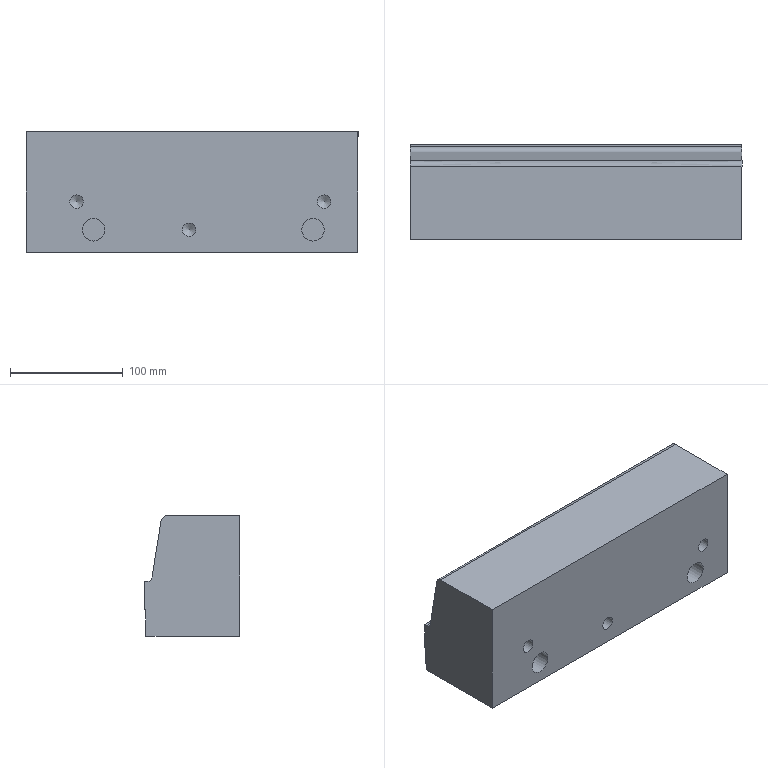Part | NX | features solid 2 | 1 solid | 22 faces | box 295 x 84.706 x 107.133 mm | volume 2449050 mm3 | plane 9 | cylinder 6 | spline 4 | cone 3 | commonest cylinder face diameters 12 x3 20 x2 10 x1
STEP:
#1=CARTESIAN_POINT('',(75.,-76.708,-50.));
#2=VERTEX_POINT('',#1);
#3=CARTESIAN_POINT('',(370.,-76.709,-50.));
#4=VERTEX_POINT('',#3);
#5=CARTESIAN_POINT('',(75.,-76.708,-50.));
#6=CARTESIAN_POINT('',(173.333,-76.71,-50.));
#7=CARTESIAN_POINT('',(271.667,-76.709,-50.));
#8=CARTESIAN_POINT('',(370.,-76.709,-50.));
#9=B_SPLINE_CURVE_WITH_KNOTS('',3,(#5,#6,#7,#8),.UNSPECIFIED.,.F.,.F.,(4,4),(0.1723,0.4673),.UNSPECIFIED.);
#10=EDGE_CURVE('',#2,#4,#9,.T.);
#11=ORIENTED_EDGE('',*,*,#10,.F.);
#12=CARTESIAN_POINT('',(75.,-76.507,-26.5));
#13=VERTEX_POINT('',#12);
#14=CARTESIAN_POINT('',(75.,-76.608,-38.267));
#15=DIRECTION('',(0.,-0.008536,-1.));
#16=VECTOR('',#15,1000.);
#17=LINE('',#14,#16);
#18=EDGE_CURVE('',#2,#13,#17,.F.);
#19=ORIENTED_EDGE('',*,*,#18,.T.);
#20=CARTESIAN_POINT('',(370.,-76.508,-26.5));
#21=VERTEX_POINT('',#20);
#22=CARTESIAN_POINT('',(75.,-76.507,-26.5));
#23=CARTESIAN_POINT('',(173.333,-76.509,-26.5));
#24=CARTESIAN_POINT('',(271.667,-76.508,-26.5));
#25=CARTESIAN_POINT('',(370.,-76.508,-26.5));
#26=B_SPLINE_CURVE_WITH_KNOTS('',3,(#22,#23,#24,#25),.UNSPECIFIED.,.F.,.F.,(4,4),(0.1378,0.4328),.UNSPECIFIED.);
#27=EDGE_CURVE('',#13,#21,#26,.T.);
#28=ORIENTED_EDGE('',*,*,#27,.T.);
#29=CARTESIAN_POINT('',(370.,-76.608,-38.267));
#30=DIRECTION('',(0.,-0.008536,-1.));
#31=VECTOR('',#30,1000.);
#32=LINE('',#29,#31);
#33=EDGE_CURVE('',#4,#21,#32,.F.);
#34=ORIENTED_EDGE('',*,*,#33,.F.);
#35=EDGE_LOOP('',(#11,#19,#28,#34));
#36=FACE_BOUND('',#35,.T.);
#37=CARTESIAN_POINT('',(75.,-76.507,-26.5));
#38=CARTESIAN_POINT('',(75.,-76.708,-50.));
#39=CARTESIAN_POINT('',(173.333,-76.509,-26.5));
#40=CARTESIAN_POINT('',(173.333,-76.71,-50.));
#41=CARTESIAN_POINT('',(271.667,-76.508,-26.5));
#42=CARTESIAN_POINT('',(271.667,-76.709,-50.));
#43=CARTESIAN_POINT('',(370.,-76.508,-26.5));
#44=CARTESIAN_POINT('',(370.,-76.709,-50.));
#45=B_SPLINE_SURFACE_WITH_KNOTS('',3,1,((#37,#38),(#39,#40),(#41,#42),(#43,#44)),.SURF_OF_LINEAR_EXTRUSION.,.F.,.F.,.F.,(4,4),(2,2),(0.5716,0.7876),(0.,1.),.PIECEWISE_BEZIER_KNOTS.);
#46=ADVANCED_FACE('',(#36),#45,.T.);
#47=ORIENTED_EDGE('',*,*,#33,.T.);
#48=CARTESIAN_POINT('',(370.,-75.295,-26.51));
#49=VERTEX_POINT('',#48);
#50=CARTESIAN_POINT('',(370.,-75.914,-26.505));
#51=DIRECTION('',(0.,-1.,0.008536));
#52=VECTOR('',#51,1000.);
#53=LINE('',#50,#52);
#54=EDGE_CURVE('',#49,#21,#53,.T.);
#55=ORIENTED_EDGE('',*,*,#54,.F.);
#56=CARTESIAN_POINT('',(370.,-75.295,-1.509));
#57=VERTEX_POINT('',#56);
#58=CARTESIAN_POINT('',(370.,-75.295,-14.009));
#59=DIRECTION('',(0.,0.,-1.));
#60=VECTOR('',#59,1000.);
#61=LINE('',#58,#60);
#62=EDGE_CURVE('',#57,#49,#61,.T.);
#63=ORIENTED_EDGE('',*,*,#62,.F.);
#64=CARTESIAN_POINT('',(370.,-77.294,-1.492));
#65=VERTEX_POINT('',#64);
#66=CARTESIAN_POINT('',(370.,47.797,-2.56));
#67=DIRECTION('',(0.,1.,-0.008536));
#68=VECTOR('',#67,1000.);
#69=LINE('',#66,#68);
#70=EDGE_CURVE('',#65,#57,#69,.T.);
#71=ORIENTED_EDGE('',*,*,#70,.F.);
#72=CARTESIAN_POINT('',(370.,-82.189,2.72));
#73=VERTEX_POINT('',#72);
#74=CARTESIAN_POINT('',(370.,-77.252,3.508));
#75=DIRECTION('',(-1.,0.,0.));
#76=DIRECTION('',(0.,0.,1.));
#77=AXIS2_PLACEMENT_3D('',#74,#75,#76);
#78=CIRCLE('',#77,5.);
#79=EDGE_CURVE('',#73,#65,#78,.F.);
#80=ORIENTED_EDGE('',*,*,#79,.F.);
#81=CARTESIAN_POINT('',(370.,-90.197,52.92));
#82=VERTEX_POINT('',#81);
#83=CARTESIAN_POINT('',(370.,-86.499,29.736));
#84=DIRECTION('',(0.,0.1575,-0.9875));
#85=VECTOR('',#84,1000.);
#86=LINE('',#83,#85);
#87=EDGE_CURVE('',#82,#73,#86,.T.);
#88=ORIENTED_EDGE('',*,*,#87,.F.);
#89=CARTESIAN_POINT('',(370.,-95.134,57.133));
#90=VERTEX_POINT('',#89);
#91=CARTESIAN_POINT('',(370.,-95.134,52.133));
#92=DIRECTION('',(-1.,0.,0.));
#93=DIRECTION('',(0.,0.,1.));
#94=AXIS2_PLACEMENT_3D('',#91,#92,#93);
#95=CIRCLE('',#94,5.);
#96=EDGE_CURVE('',#82,#90,#95,.F.);
#97=ORIENTED_EDGE('',*,*,#96,.T.);
#98=CARTESIAN_POINT('',(370.,-160.,57.133));
#99=VERTEX_POINT('',#98);
#100=CARTESIAN_POINT('',(370.,-90.869,57.133));
#101=DIRECTION('',(0.,-1.,0.));
#102=VECTOR('',#101,1000.);
#103=LINE('',#100,#102);
#104=EDGE_CURVE('',#90,#99,#103,.T.);
#105=ORIENTED_EDGE('',*,*,#104,.T.);
#106=CARTESIAN_POINT('',(370.,-160.,-50.));
#107=VERTEX_POINT('',#106);
#108=CARTESIAN_POINT('',(370.,-160.,200.));
#109=DIRECTION('',(0.,0.,1.));
#110=VECTOR('',#109,1000.);
#111=LINE('',#108,#110);
#112=EDGE_CURVE('',#107,#99,#111,.T.);
#113=ORIENTED_EDGE('',*,*,#112,.F.);
#114=CARTESIAN_POINT('',(370.,361.,-50.));
#115=DIRECTION('',(0.,-1.,0.));
#116=VECTOR('',#115,1000.);
#117=LINE('',#114,#116);
#118=EDGE_CURVE('',#107,#4,#117,.F.);
#119=ORIENTED_EDGE('',*,*,#118,.T.);
#120=EDGE_LOOP('',(#47,#55,#63,#71,#80,#88,#97,#105,#113,#119));
#121=FACE_BOUND('',#120,.T.);
#122=CARTESIAN_POINT('',(370.,361.,0.));
#123=DIRECTION('',(-1.,0.,0.));
#124=DIRECTION('',(0.,0.,1.));
#125=AXIS2_PLACEMENT_3D('',#122,#123,#124);
#126=PLANE('',#125);
#127=ADVANCED_FACE('',(#121),#126,.F.);
#128=CARTESIAN_POINT('',(75.,-160.,-50.));
#129=VERTEX_POINT('',#128);
#130=CARTESIAN_POINT('',(75.,-159.,-50.));
#131=DIRECTION('',(0.,1.,0.));
#132=VECTOR('',#131,1000.);
#133=LINE('',#130,#132);
#134=EDGE_CURVE('',#129,#2,#133,.T.);
#135=ORIENTED_EDGE('',*,*,#134,.T.);
#136=ORIENTED_EDGE('',*,*,#10,.T.);
#137=ORIENTED_EDGE('',*,*,#118,.F.);
#138=CARTESIAN_POINT('',(-571.479,-160.,-50.));
#139=DIRECTION('',(1.,0.,0.));
#140=VECTOR('',#139,1000.);
#141=LINE('',#138,#140);
#142=EDGE_CURVE('',#129,#107,#141,.T.);
#143=ORIENTED_EDGE('',*,*,#142,.F.);
#144=EDGE_LOOP('',(#135,#136,#137,#143));
#145=FACE_BOUND('',#144,.T.);
#146=CARTESIAN_POINT('',(-571.479,-74.471,-50.));
#147=DIRECTION('',(0.,0.,-1.));
#148=DIRECTION('',(-1.,0.,0.));
#149=AXIS2_PLACEMENT_3D('',#146,#147,#148);
#150=PLANE('',#149);
#151=ADVANCED_FACE('',(#145),#150,.T.);
#152=ORIENTED_EDGE('',*,*,#142,.T.);
#153=ORIENTED_EDGE('',*,*,#112,.T.);
#154=CARTESIAN_POINT('',(75.,-160.,57.133));
#155=VERTEX_POINT('',#154);
#156=CARTESIAN_POINT('',(-705.,-160.,57.133));
#157=DIRECTION('',(1.,0.,0.));
#158=VECTOR('',#157,1000.);
#159=LINE('',#156,#158);
#160=EDGE_CURVE('',#155,#99,#159,.T.);
#161=ORIENTED_EDGE('',*,*,#160,.F.);
#162=CARTESIAN_POINT('',(75.,-160.,200.));
#163=DIRECTION('',(0.,0.,1.));
#164=VECTOR('',#163,1000.);
#165=LINE('',#162,#164);
#166=EDGE_CURVE('',#129,#155,#165,.T.);
#167=ORIENTED_EDGE('',*,*,#166,.F.);
#168=EDGE_LOOP('',(#152,#153,#161,#167));
#169=FACE_BOUND('',#168,.T.);
#170=CARTESIAN_POINT('',(340.,-160.,1.));
#171=VERTEX_POINT('',#170);
#172=CARTESIAN_POINT('',(340.,-160.,-5.));
#173=DIRECTION('',(0.,1.,0.));
#174=DIRECTION('',(0.,0.,1.));
#175=AXIS2_PLACEMENT_3D('',#172,#173,#174);
#176=CIRCLE('',#175,6.);
#177=EDGE_CURVE('',#171,#171,#176,.T.);
#178=ORIENTED_EDGE('',*,*,#177,.T.);
#179=EDGE_LOOP('',(#178));
#180=FACE_BOUND('',#179,.T.);
#181=CARTESIAN_POINT('',(220.,-160.,-24.));
#182=VERTEX_POINT('',#181);
#183=CARTESIAN_POINT('',(220.,-160.,-30.));
#184=DIRECTION('',(0.,1.,0.));
#185=DIRECTION('',(0.,0.,1.));
#186=AXIS2_PLACEMENT_3D('',#183,#184,#185);
#187=CIRCLE('',#186,6.);
#188=EDGE_CURVE('',#182,#182,#187,.T.);
#189=ORIENTED_EDGE('',*,*,#188,.T.);
#190=EDGE_LOOP('',(#189));
#191=FACE_BOUND('',#190,.T.);
#192=CARTESIAN_POINT('',(120.,-160.,1.));
#193=VERTEX_POINT('',#192);
#194=CARTESIAN_POINT('',(120.,-160.,-5.));
#195=DIRECTION('',(0.,1.,0.));
#196=DIRECTION('',(0.,0.,1.));
#197=AXIS2_PLACEMENT_3D('',#194,#195,#196);
#198=CIRCLE('',#197,6.);
#199=EDGE_CURVE('',#193,#193,#198,.T.);
#200=ORIENTED_EDGE('',*,*,#199,.T.);
#201=EDGE_LOOP('',(#200));
#202=FACE_BOUND('',#201,.T.);
#203=CARTESIAN_POINT('',(330.,-160.,-20.));
#204=VERTEX_POINT('',#203);
#205=CARTESIAN_POINT('',(330.,-160.,-30.));
#206=DIRECTION('',(0.,1.,0.));
#207=DIRECTION('',(0.,0.,1.));
#208=AXIS2_PLACEMENT_3D('',#205,#206,#207);
#209=CIRCLE('',#208,10.);
#210=EDGE_CURVE('',#204,#204,#209,.T.);
#211=ORIENTED_EDGE('',*,*,#210,.T.);
#212=EDGE_LOOP('',(#211));
#213=FACE_BOUND('',#212,.T.);
#214=CARTESIAN_POINT('',(135.,-160.,-20.));
#215=VERTEX_POINT('',#214);
#216=CARTESIAN_POINT('',(135.,-160.,-30.));
#217=DIRECTION('',(0.,1.,0.));
#218=DIRECTION('',(0.,0.,1.));
#219=AXIS2_PLACEMENT_3D('',#216,#217,#218);
#220=CIRCLE('',#219,10.);
#221=EDGE_CURVE('',#215,#215,#220,.T.);
#222=ORIENTED_EDGE('',*,*,#221,.T.);
#223=EDGE_LOOP('',(#222));
#224=FACE_BOUND('',#223,.T.);
#225=CARTESIAN_POINT('',(-705.,-160.,200.));
#226=DIRECTION('',(0.,1.,0.));
#227=DIRECTION('',(0.,0.,1.));
#228=AXIS2_PLACEMENT_3D('',#225,#226,#227);
#229=PLANE('',#228);
#230=ADVANCED_FACE('',(#169,#180,#191,#202,#213,#224),#229,.F.);
#231=ORIENTED_EDGE('',*,*,#96,.F.);
#232=CARTESIAN_POINT('',(75.,-90.197,52.92));
#233=VERTEX_POINT('',#232);
#234=CARTESIAN_POINT('',(75.,-90.197,52.92));
#235=CARTESIAN_POINT('',(173.333,-90.197,52.92));
#236=CARTESIAN_POINT('',(271.667,-90.197,52.92));
#237=CARTESIAN_POINT('',(370.,-90.197,52.92));
#238=B_SPLINE_CURVE_WITH_KNOTS('',3,(#234,#235,#236,#237),.UNSPECIFIED.,.F.,.F.,(4,4),(0.2731,0.5681),.UNSPECIFIED.);
#239=EDGE_CURVE('',#233,#82,#238,.T.);
#240=ORIENTED_EDGE('',*,*,#239,.F.);
#241=CARTESIAN_POINT('',(75.,-95.134,57.133));
#242=VERTEX_POINT('',#241);
#243=CARTESIAN_POINT('',(75.,-95.134,52.133));
#244=DIRECTION('',(-1.,0.,0.));
#245=DIRECTION('',(0.,0.,1.));
#246=AXIS2_PLACEMENT_3D('',#243,#244,#245);
#247=CIRCLE('',#246,5.);
#248=EDGE_CURVE('',#233,#242,#247,.F.);
#249=ORIENTED_EDGE('',*,*,#248,.T.);
#250=CARTESIAN_POINT('',(370.,-95.134,57.133));
#251=CARTESIAN_POINT('',(271.667,-95.134,57.133));
#252=CARTESIAN_POINT('',(173.333,-95.134,57.133));
#253=CARTESIAN_POINT('',(75.,-95.134,57.133));
#254=B_SPLINE_CURVE_WITH_KNOTS('',3,(#250,#251,#252,#253),.UNSPECIFIED.,.F.,.F.,(4,4),(0.3736,0.6686),.UNSPECIFIED.);
#255=EDGE_CURVE('',#90,#242,#254,.T.);
#256=ORIENTED_EDGE('',*,*,#255,.F.);
#257=EDGE_LOOP('',(#231,#240,#249,#256));
#258=FACE_BOUND('',#257,.T.);
#259=CARTESIAN_POINT('',(370.,-90.197,52.92));
#260=CARTESIAN_POINT('',(370.,-90.869,57.133));
#261=CARTESIAN_POINT('',(370.,-95.134,57.133));
#262=CARTESIAN_POINT('',(271.667,-90.197,52.92));
#263=CARTESIAN_POINT('',(271.667,-90.869,57.133));
#264=CARTESIAN_POINT('',(271.667,-95.134,57.133));
#265=CARTESIAN_POINT('',(173.333,-90.197,52.92));
#266=CARTESIAN_POINT('',(173.333,-90.869,57.133));
#267=CARTESIAN_POINT('',(173.333,-95.134,57.133));
#268=CARTESIAN_POINT('',(75.,-90.197,52.92));
#269=CARTESIAN_POINT('',(75.,-90.869,57.133));
#270=CARTESIAN_POINT('',(75.,-95.134,57.133));
#271=(BOUNDED_SURFACE()B_SPLINE_SURFACE(3,2,((#259,#260,#261),(#262,#263,#264),(#265,#266,#267),(#268,#269,#270)),.UNSPECIFIED.,.F.,.F.,.F.)B_SPLINE_SURFACE_WITH_KNOTS((4,4),(3,3),(0.4893,0.7843),(0.,1.),.PIECEWISE_BEZIER_KNOTS.)GEOMETRIC_REPRESENTATION_ITEM()RATIONAL_B_SPLINE_SURFACE(((1.,0.7608,1.),(1.,0.7608,1.),(1.,0.7608,1.),(1.,0.7608,1.)))REPRESENTATION_ITEM('')SURFACE());
#272=ADVANCED_FACE('',(#258),#271,.T.);
#273=ORIENTED_EDGE('',*,*,#239,.T.);
#274=ORIENTED_EDGE('',*,*,#87,.T.);
#275=CARTESIAN_POINT('',(75.,-82.189,2.72));
#276=VERTEX_POINT('',#275);
#277=CARTESIAN_POINT('',(75.,-82.189,2.72));
#278=CARTESIAN_POINT('',(173.333,-82.189,2.72));
#279=CARTESIAN_POINT('',(271.667,-82.189,2.72));
#280=CARTESIAN_POINT('',(370.,-82.189,2.72));
#281=B_SPLINE_CURVE_WITH_KNOTS('',3,(#277,#278,#279,#280),.UNSPECIFIED.,.F.,.F.,(4,4),(0.3113,0.6615),.UNSPECIFIED.);
#282=EDGE_CURVE('',#276,#73,#281,.T.);
#283=ORIENTED_EDGE('',*,*,#282,.F.);
#284=CARTESIAN_POINT('',(75.,-86.499,29.736));
#285=DIRECTION('',(0.,0.1575,-0.9875));
#286=VECTOR('',#285,1000.);
#287=LINE('',#284,#286);
#288=EDGE_CURVE('',#233,#276,#287,.T.);
#289=ORIENTED_EDGE('',*,*,#288,.F.);
#290=EDGE_LOOP('',(#273,#274,#283,#289));
#291=FACE_BOUND('',#290,.T.);
#292=CARTESIAN_POINT('',(808.196,-81.695,-0.3814));
#293=CARTESIAN_POINT('',(-199.284,-81.695,-0.3814));
#294=CARTESIAN_POINT('',(808.196,-91.303,59.853));
#295=CARTESIAN_POINT('',(-199.284,-91.303,59.853));
#296=B_SPLINE_SURFACE_WITH_KNOTS('',1,1,((#292,#293),(#294,#295)),.PLANE_SURF.,.F.,.F.,.F.,(2,2),(2,2),(-0.06964,1.283),(-0.1722,1.),.UNSPECIFIED.);
#297=ADVANCED_FACE('',(#291),#296,.F.);
#298=ORIENTED_EDGE('',*,*,#282,.T.);
#299=ORIENTED_EDGE('',*,*,#79,.T.);
#300=CARTESIAN_POINT('',(75.,-77.294,-1.492));
#301=VERTEX_POINT('',#300);
#302=CARTESIAN_POINT('',(370.,-77.294,-1.492));
#303=CARTESIAN_POINT('',(271.667,-77.294,-1.492));
#304=CARTESIAN_POINT('',(173.333,-77.294,-1.492));
#305=CARTESIAN_POINT('',(75.,-77.294,-1.492));
#306=B_SPLINE_CURVE_WITH_KNOTS('',3,(#302,#303,#304,#305),.UNSPECIFIED.,.F.,.F.,(4,4),(0.3388,0.6888),.UNSPECIFIED.);
#307=EDGE_CURVE('',#65,#301,#306,.T.);
#308=ORIENTED_EDGE('',*,*,#307,.T.);
#309=CARTESIAN_POINT('',(75.,-77.252,3.508));
#310=DIRECTION('',(-1.,0.,0.));
#311=DIRECTION('',(0.,0.,1.));
#312=AXIS2_PLACEMENT_3D('',#309,#310,#311);
#313=CIRCLE('',#312,5.);
#314=EDGE_CURVE('',#276,#301,#313,.F.);
#315=ORIENTED_EDGE('',*,*,#314,.F.);
#316=EDGE_LOOP('',(#298,#299,#308,#315));
#317=FACE_BOUND('',#316,.T.);
#318=CARTESIAN_POINT('',(6000655.556,-77.252,3.508));
#319=DIRECTION('',(-1.,0.,0.));
#320=DIRECTION('',(0.,-0.1575,0.9875));
#321=AXIS2_PLACEMENT_3D('',#318,#319,#320);
#322=CYLINDRICAL_SURFACE('',#321,5.);
#323=ADVANCED_FACE('',(#317),#322,.F.);
#324=ORIENTED_EDGE('',*,*,#307,.F.);
#325=ORIENTED_EDGE('',*,*,#70,.T.);
#326=CARTESIAN_POINT('',(75.,-75.294,-1.509));
#327=VERTEX_POINT('',#326);
#328=CARTESIAN_POINT('',(75.,-75.294,-1.509));
#329=CARTESIAN_POINT('',(173.333,-75.295,-1.509));
#330=CARTESIAN_POINT('',(271.667,-75.295,-1.509));
#331=CARTESIAN_POINT('',(370.,-75.295,-1.509));
#332=B_SPLINE_CURVE_WITH_KNOTS('',3,(#328,#329,#330,#331),.UNSPECIFIED.,.F.,.F.,(4,4),(0.4725,0.7675),.UNSPECIFIED.);
#333=EDGE_CURVE('',#327,#57,#332,.T.);
#334=ORIENTED_EDGE('',*,*,#333,.F.);
#335=CARTESIAN_POINT('',(75.,47.797,-2.56));
#336=DIRECTION('',(0.,1.,-0.008536));
#337=VECTOR('',#336,1000.);
#338=LINE('',#335,#337);
#339=EDGE_CURVE('',#301,#327,#338,.T.);
#340=ORIENTED_EDGE('',*,*,#339,.F.);
#341=EDGE_LOOP('',(#324,#325,#334,#340));
#342=FACE_BOUND('',#341,.T.);
#343=CARTESIAN_POINT('',(35.495,47.797,-2.56));
#344=DIRECTION('',(0.,-0.008536,-1.));
#345=DIRECTION('',(0.,-1.,0.008536));
#346=AXIS2_PLACEMENT_3D('',#343,#344,#345);
#347=PLANE('',#346);
#348=ADVANCED_FACE('',(#342),#347,.F.);
#349=ORIENTED_EDGE('',*,*,#333,.T.);
#350=ORIENTED_EDGE('',*,*,#62,.T.);
#351=CARTESIAN_POINT('',(75.,-75.294,-26.51));
#352=VERTEX_POINT('',#351);
#353=CARTESIAN_POINT('',(370.,-75.295,-26.51));
#354=CARTESIAN_POINT('',(271.667,-75.295,-26.51));
#355=CARTESIAN_POINT('',(173.333,-75.295,-26.51));
#356=CARTESIAN_POINT('',(75.,-75.294,-26.51));
#357=B_SPLINE_CURVE_WITH_KNOTS('',3,(#353,#354,#355,#356),.UNSPECIFIED.,.F.,.F.,(4,4),(0.29,0.585),.UNSPECIFIED.);
#358=EDGE_CURVE('',#49,#352,#357,.T.);
#359=ORIENTED_EDGE('',*,*,#358,.T.);
#360=CARTESIAN_POINT('',(75.,-75.294,-14.008));
#361=DIRECTION('',(0.,0.,-1.));
#362=VECTOR('',#361,1000.);
#363=LINE('',#360,#362);
#364=EDGE_CURVE('',#327,#352,#363,.T.);
#365=ORIENTED_EDGE('',*,*,#364,.F.);
#366=EDGE_LOOP('',(#349,#350,#359,#365));
#367=FACE_BOUND('',#366,.T.);
#368=CARTESIAN_POINT('',(370.,-75.295,-1.509));
#369=CARTESIAN_POINT('',(370.,-75.295,-26.51));
#370=CARTESIAN_POINT('',(271.667,-75.295,-1.509));
#371=CARTESIAN_POINT('',(271.667,-75.295,-26.51));
#372=CARTESIAN_POINT('',(173.333,-75.295,-1.509));
#373=CARTESIAN_POINT('',(173.333,-75.295,-26.51));
#374=CARTESIAN_POINT('',(75.,-75.294,-1.509));
#375=CARTESIAN_POINT('',(75.,-75.294,-26.51));
#376=B_SPLINE_SURFACE_WITH_KNOTS('',3,1,((#368,#369),(#370,#371),(#372,#373),(#374,#375)),.SURF_OF_LINEAR_EXTRUSION.,.F.,.F.,.F.,(4,4),(2,2),(0.2124,0.4284),(0.,1.),.PIECEWISE_BEZIER_KNOTS.);
#377=ADVANCED_FACE('',(#367),#376,.F.);
#378=ORIENTED_EDGE('',*,*,#27,.F.);
#379=CARTESIAN_POINT('',(75.,-75.914,-26.505));
#380=DIRECTION('',(0.,-1.,0.008536));
#381=VECTOR('',#380,1000.);
#382=LINE('',#379,#381);
#383=EDGE_CURVE('',#352,#13,#382,.T.);
#384=ORIENTED_EDGE('',*,*,#383,.F.);
#385=ORIENTED_EDGE('',*,*,#358,.F.);
#386=ORIENTED_EDGE('',*,*,#54,.T.);
#387=EDGE_LOOP('',(#378,#384,#385,#386));
#388=FACE_BOUND('',#387,.T.);
#389=CARTESIAN_POINT('',(-437.652,-75.914,-26.505));
#390=DIRECTION('',(0.,0.008536,1.));
#391=DIRECTION('',(0.,-1.,0.008536));
#392=AXIS2_PLACEMENT_3D('',#389,#390,#391);
#393=PLANE('',#392);
#394=ADVANCED_FACE('',(#388),#393,.F.);
#395=ORIENTED_EDGE('',*,*,#383,.T.);
#396=ORIENTED_EDGE('',*,*,#18,.F.);
#397=ORIENTED_EDGE('',*,*,#134,.F.);
#398=ORIENTED_EDGE('',*,*,#166,.T.);
#399=CARTESIAN_POINT('',(75.,-90.869,57.133));
#400=DIRECTION('',(0.,-1.,0.));
#401=VECTOR('',#400,1000.);
#402=LINE('',#399,#401);
#403=EDGE_CURVE('',#242,#155,#402,.T.);
#404=ORIENTED_EDGE('',*,*,#403,.F.);
#405=ORIENTED_EDGE('',*,*,#248,.F.);
#406=ORIENTED_EDGE('',*,*,#288,.T.);
#407=ORIENTED_EDGE('',*,*,#314,.T.);
#408=ORIENTED_EDGE('',*,*,#339,.T.);
#409=ORIENTED_EDGE('',*,*,#364,.T.);
#410=EDGE_LOOP('',(#395,#396,#397,#398,#404,#405,#406,#407,#408,#409));
#411=FACE_BOUND('',#410,.T.);
#412=CARTESIAN_POINT('',(75.,361.,0.));
#413=DIRECTION('',(-1.,0.,0.));
#414=DIRECTION('',(0.,0.,1.));
#415=AXIS2_PLACEMENT_3D('',#412,#413,#414);
#416=PLANE('',#415);
#417=ADVANCED_FACE('',(#411),#416,.T.);
#418=ORIENTED_EDGE('',*,*,#104,.F.);
#419=ORIENTED_EDGE('',*,*,#255,.T.);
#420=ORIENTED_EDGE('',*,*,#403,.T.);
#421=ORIENTED_EDGE('',*,*,#160,.T.);
#422=EDGE_LOOP('',(#418,#419,#420,#421));
#423=FACE_BOUND('',#422,.T.);
#424=CARTESIAN_POINT('',(743.607,-90.869,57.133));
#425=DIRECTION('',(0.,0.,1.));
#426=DIRECTION('',(1.,0.,0.));
#427=AXIS2_PLACEMENT_3D('',#424,#425,#426);
#428=PLANE('',#427);
#429=ADVANCED_FACE('',(#423),#428,.T.);
#430=CARTESIAN_POINT('',(340.,-129.,1.));
#431=VERTEX_POINT('',#430);
#432=CARTESIAN_POINT('',(340.,-129.,-5.));
#433=DIRECTION('',(0.,1.,0.));
#434=DIRECTION('',(0.,0.,1.));
#435=AXIS2_PLACEMENT_3D('',#432,#433,#434);
#436=CIRCLE('',#435,6.);
#437=EDGE_CURVE('',#431,#431,#436,.T.);
#438=ORIENTED_EDGE('',*,*,#437,.F.);
#439=EDGE_LOOP('',(#438));
#440=FACE_BOUND('',#439,.T.);
#441=CARTESIAN_POINT('',(340.,-125.395,-5.));
#442=VERTEX_POINT('',#441);
#443=VERTEX_LOOP('',#442);
#444=FACE_BOUND('',#443,.T.);
#445=CARTESIAN_POINT('',(340.,-129.,-5.));
#446=DIRECTION('',(0.,-1.,0.));
#447=DIRECTION('',(0.,0.,-1.));
#448=AXIS2_PLACEMENT_3D('',#445,#446,#447);
#449=CONICAL_SURFACE('',#448,6.,1.03);
#450=ADVANCED_FACE('',(#440,#444),#449,.F.);
#451=ORIENTED_EDGE('',*,*,#437,.T.);
#452=EDGE_LOOP('',(#451));
#453=FACE_BOUND('',#452,.T.);
#454=ORIENTED_EDGE('',*,*,#177,.F.);
#455=EDGE_LOOP('',(#454));
#456=FACE_BOUND('',#455,.T.);
#457=CARTESIAN_POINT('',(340.,-159.,-5.));
#458=DIRECTION('',(0.,1.,0.));
#459=DIRECTION('',(0.,0.,1.));
#460=AXIS2_PLACEMENT_3D('',#457,#458,#459);
#461=CYLINDRICAL_SURFACE('',#460,6.);
#462=ADVANCED_FACE('',(#453,#456),#461,.F.);
#463=CARTESIAN_POINT('',(220.,-129.,-24.));
#464=VERTEX_POINT('',#463);
#465=CARTESIAN_POINT('',(220.,-129.,-30.));
#466=DIRECTION('',(0.,1.,0.));
#467=DIRECTION('',(0.,0.,1.));
#468=AXIS2_PLACEMENT_3D('',#465,#466,#467);
#469=CIRCLE('',#468,6.);
#470=EDGE_CURVE('',#464,#464,#469,.T.);
#471=ORIENTED_EDGE('',*,*,#470,.F.);
#472=EDGE_LOOP('',(#471));
#473=FACE_BOUND('',#472,.T.);
#474=CARTESIAN_POINT('',(220.,-125.395,-30.));
#475=VERTEX_POINT('',#474);
#476=VERTEX_LOOP('',#475);
#477=FACE_BOUND('',#476,.T.);
#478=CARTESIAN_POINT('',(220.,-129.,-30.));
#479=DIRECTION('',(0.,-1.,0.));
#480=DIRECTION('',(0.,0.,-1.));
#481=AXIS2_PLACEMENT_3D('',#478,#479,#480);
#482=CONICAL_SURFACE('',#481,6.,1.03);
#483=ADVANCED_FACE('',(#473,#477),#482,.F.);
#484=ORIENTED_EDGE('',*,*,#470,.T.);
#485=EDGE_LOOP('',(#484));
#486=FACE_BOUND('',#485,.T.);
#487=ORIENTED_EDGE('',*,*,#188,.F.);
#488=EDGE_LOOP('',(#487));
#489=FACE_BOUND('',#488,.T.);
#490=CARTESIAN_POINT('',(220.,-159.,-30.));
#491=DIRECTION('',(0.,1.,0.));
#492=DIRECTION('',(0.,0.,1.));
#493=AXIS2_PLACEMENT_3D('',#490,#491,#492);
#494=CYLINDRICAL_SURFACE('',#493,6.);
#495=ADVANCED_FACE('',(#486,#489),#494,.F.);
#496=CARTESIAN_POINT('',(120.,-129.,1.));
#497=VERTEX_POINT('',#496);
#498=CARTESIAN_POINT('',(120.,-129.,-5.));
#499=DIRECTION('',(0.,1.,0.));
#500=DIRECTION('',(0.,0.,1.));
#501=AXIS2_PLACEMENT_3D('',#498,#499,#500);
#502=CIRCLE('',#501,6.);
#503=EDGE_CURVE('',#497,#497,#502,.T.);
#504=ORIENTED_EDGE('',*,*,#503,.F.);
#505=EDGE_LOOP('',(#504));
#506=FACE_BOUND('',#505,.T.);
#507=CARTESIAN_POINT('',(120.,-125.395,-5.));
#508=VERTEX_POINT('',#507);
#509=VERTEX_LOOP('',#508);
#510=FACE_BOUND('',#509,.T.);
#511=CARTESIAN_POINT('',(120.,-129.,-5.));
#512=DIRECTION('',(0.,-1.,0.));
#513=DIRECTION('',(0.,0.,-1.));
#514=AXIS2_PLACEMENT_3D('',#511,#512,#513);
#515=CONICAL_SURFACE('',#514,6.,1.03);
#516=ADVANCED_FACE('',(#506,#510),#515,.F.);
#517=ORIENTED_EDGE('',*,*,#503,.T.);
#518=EDGE_LOOP('',(#517));
#519=FACE_BOUND('',#518,.T.);
#520=ORIENTED_EDGE('',*,*,#199,.F.);
#521=EDGE_LOOP('',(#520));
#522=FACE_BOUND('',#521,.T.);
#523=CARTESIAN_POINT('',(120.,-159.,-5.));
#524=DIRECTION('',(0.,1.,0.));
#525=DIRECTION('',(0.,0.,1.));
#526=AXIS2_PLACEMENT_3D('',#523,#524,#525);
#527=CYLINDRICAL_SURFACE('',#526,6.);
#528=ADVANCED_FACE('',(#519,#522),#527,.F.);
#529=CARTESIAN_POINT('',(330.,-129.,-20.));
#530=VERTEX_POINT('',#529);
#531=CARTESIAN_POINT('',(330.,-129.,-30.));
#532=DIRECTION('',(0.,1.,0.));
#533=DIRECTION('',(0.,0.,1.));
#534=AXIS2_PLACEMENT_3D('',#531,#532,#533);
#535=CIRCLE('',#534,10.);
#536=EDGE_CURVE('',#530,#530,#535,.T.);
#537=ORIENTED_EDGE('',*,*,#536,.T.);
#538=EDGE_LOOP('',(#537));
#539=FACE_BOUND('',#538,.T.);
#540=ORIENTED_EDGE('',*,*,#210,.F.);
#541=EDGE_LOOP('',(#540));
#542=FACE_BOUND('',#541,.T.);
#543=CARTESIAN_POINT('',(330.,-159.,-30.));
#544=DIRECTION('',(0.,1.,0.));
#545=DIRECTION('',(0.,0.,1.));
#546=AXIS2_PLACEMENT_3D('',#543,#544,#545);
#547=CYLINDRICAL_SURFACE('',#546,10.);
#548=ADVANCED_FACE('',(#539,#542),#547,.F.);
#549=ORIENTED_EDGE('',*,*,#536,.F.);
#550=EDGE_LOOP('',(#549));
#551=FACE_BOUND('',#550,.T.);
#552=CARTESIAN_POINT('',(330.,-129.,-30.));
#553=DIRECTION('',(0.,1.,0.));
#554=DIRECTION('',(0.,0.,1.));
#555=AXIS2_PLACEMENT_3D('',#552,#553,#554);
#556=PLANE('',#555);
#557=ADVANCED_FACE('',(#551),#556,.F.);
#558=CARTESIAN_POINT('',(135.,-129.,-20.));
#559=VERTEX_POINT('',#558);
#560=CARTESIAN_POINT('',(135.,-129.,-30.));
#561=DIRECTION('',(0.,1.,0.));
#562=DIRECTION('',(0.,0.,1.));
#563=AXIS2_PLACEMENT_3D('',#560,#561,#562);
#564=CIRCLE('',#563,10.);
#565=EDGE_CURVE('',#559,#559,#564,.T.);
#566=ORIENTED_EDGE('',*,*,#565,.T.);
#567=EDGE_LOOP('',(#566));
#568=FACE_BOUND('',#567,.T.);
#569=ORIENTED_EDGE('',*,*,#221,.F.);
#570=EDGE_LOOP('',(#569));
#571=FACE_BOUND('',#570,.T.);
#572=CARTESIAN_POINT('',(135.,-159.,-30.));
#573=DIRECTION('',(0.,1.,0.));
#574=DIRECTION('',(0.,0.,1.));
#575=AXIS2_PLACEMENT_3D('',#572,#573,#574);
#576=CYLINDRICAL_SURFACE('',#575,10.);
#577=ADVANCED_FACE('',(#568,#571),#576,.F.);
#578=ORIENTED_EDGE('',*,*,#565,.F.);
#579=EDGE_LOOP('',(#578));
#580=FACE_BOUND('',#579,.T.);
#581=CARTESIAN_POINT('',(135.,-129.,-30.));
#582=DIRECTION('',(0.,1.,0.));
#583=DIRECTION('',(0.,0.,1.));
#584=AXIS2_PLACEMENT_3D('',#581,#582,#583);
#585=PLANE('',#584);
#586=ADVANCED_FACE('',(#580),#585,.F.);
#587=CLOSED_SHELL('',(#46,#127,#151,#230,#272,#297,#323,#348,#377,#394,#417,#429,#450,#462,#483,#495,#516,#528,#548,#557,#577,#586));
#588=MANIFOLD_SOLID_BREP('',#587);
#589=(LENGTH_UNIT()NAMED_UNIT(*)SI_UNIT(.MILLI.,.METRE.));
#590=UNCERTAINTY_MEASURE_WITH_UNIT(LENGTH_MEASURE(0.0508),#589,'','');
#591=(NAMED_UNIT(*)PLANE_ANGLE_UNIT()SI_UNIT($,.RADIAN.));
#592=(NAMED_UNIT(*)SI_UNIT($,.STERADIAN.)SOLID_ANGLE_UNIT());
#593=(GEOMETRIC_REPRESENTATION_CONTEXT(3)GLOBAL_UNCERTAINTY_ASSIGNED_CONTEXT((#590))GLOBAL_UNIT_ASSIGNED_CONTEXT((#589,#591,#592))REPRESENTATION_CONTEXT('',''));
#594=ADVANCED_BREP_SHAPE_REPRESENTATION('',(#588),#593);